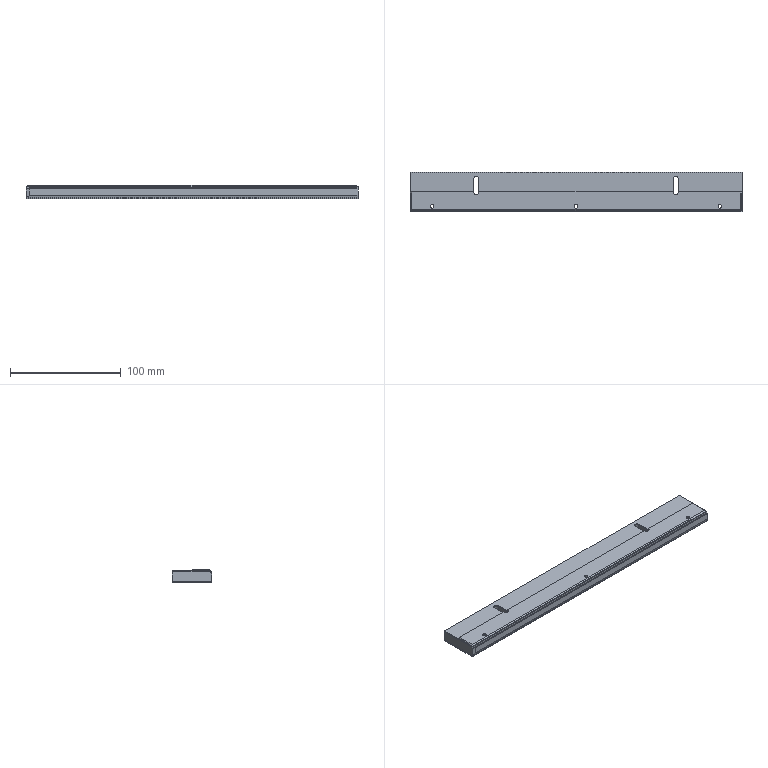CAM job | NX | 3-axis milling, drilling | part box 300 x 36 x 12 mm | stock box 305 x 41 x 15 mm
Tools:
number,name,description,diameter,corner_radius,flute_length,length,flutes
4,D4,平底铣刀-粗,4.0,0.0,25.0,75.0,2
6,D6,平底铣刀-粗,6.0,0.0,25.0,75.0,2
9,D10,平底铣刀-粗,10.0,0.0,35.0,75.0,2
11,D4-J,平底铣刀-精,4.0,0.0,50.0,75.0,2
7,D6-J,平底铣刀-精,6.0,0.0,25.0,75.0,2
10,D10-J,平底铣刀-精,10.0,0.0,35.0,75.0,2
17,D6R0.5,圆鼻刀-粗,6.0,0.5,50.0,75.0,2
2,D6倒角刀,倒角刀,6.0,0.0,3.0,25.0,2
21,M4X0.7,丝锥,3.3,0.0,35.0,50.0,2
13,ZT3.3,钻头,3.3,0.0,35.0,50.0,2
Operations:
program,operation,operation_type,tool,method,geometry_group,spindle_rpm,surface_speed,feed_per_tooth,feed_cut,feed_plunge,cut_length_mm,path_length_mm,cut_time_min,machine_time_min
D,顶面_COPY_COPY,FaceMilling,D10-J,侧刃精光-切深K-步距G,W-D,4500.0,1385.0,0.1667,1500.0,100.0,4781.035,5160.146,3.187,3.225
D,面铣自动飞面精光_COPY_COPY_COPY_1,FaceMilling,D10-J,侧刃精光-切深K-步距G,W-D,8000.0,251.327,0.0625,1000.0,100.0,2410.317,2466.317,2.41,2.416
D,底壁铣分层开粗-中_COPY_1,VolumeBased25DMillingOperation,D6,分层开粗-切深K-步距G,W-D,8000.0,150.792,0.1875,3000.0,100.0,4661.335,5306.774,1.554,1.618
D,打点-深0.8_2,Operation,D6倒角刀,NONE,W-D,8000.0,150.796,0.0312,500.0,90.0,5.4,332.808,0.0108,0.0435
D,通孔-M4螺纹底孔_2,Operation,ZT3.3,NONE,W-D,3000.0,30.536,0.05,300.0,90.0,48.0,418.008,0.16,0.197
D,钻倒角_1,Operation,D6倒角刀,METHOD,W-D,8000.0,150.796,0.0312,500.0,0.0,15.513,357.095,0.031,0.0652
D,通孔-攻牙M4_2,Operation,M4X0.7,METHOD,W-D,600.0,6.22,0.0006,0.7,90.0,42.0,406.008,60.0,60.036
D,底壁铣精光底面-中_COPY_1,VolumeBased25DMillingOperation,D6-J,精光步距切深关,W-D,8000.0,150.792,0.0625,1000.0,100.0,1838.862,1860.262,1.839,1.841
D,底壁铣精光侧面-中-选底面_COPY_1,VolumeBased25DMillingOperation,D6-J,侧刃精光-切深K-步距G,W-D,8000.0,150.792,0.0625,1000.0,100.0,312.168,334.568,0.3122,0.3144
D,底壁铣精光侧面-中_COPY,VolumeBased25DMillingOperation,D6-J,侧刃精光-切深K-步距G,W-D,8000.0,150.792,0.0625,1000.0,100.0,935.206,1617.172,0.9352,1.003
D,平面去毛刺6X45L_COPY_2,SurfaceContour,D6倒角刀,爬面_倒角-切深0-步距G,W-D,6500.0,122.519,0.1154,1500.0,100.0,753.227,1659.511,0.5022,0.5928
D,底壁铣倒角_COPY_2,VolumeBased25DMillingOperation,D6倒角刀,爬面_倒角-切深0-步距G,W-D,6500.0,122.519,0.1154,1500.0,100.0,349.496,408.896,0.233,0.2389
C,面铣自动飞面精光_COPY_COPY_COPY,FaceMilling,D10-J,侧刃精光-切深K-步距G,W-C,8000.0,251.327,0.0625,1000.0,100.0,4820.633,5253.341,4.821,4.864
C,面铣自动飞面精光_COPY_COPY,FaceMilling,D10-J,侧刃精光-切深K-步距G,W-C,8000.0,251.327,0.0625,1000.0,100.0,2410.317,2506.317,2.41,2.42
C,通腰槽粗_1,VolumeBased25DMillingOperation,D4,METHOD,W-C,10000.0,125.664,0.06,1200.0,100.0,2247.933,2645.634,1.873,1.913
C,腰槽精_1,VolumeBased25DMillingOperation,D4-J,METHOD,W-C,8000.0,100.531,0.0312,500.0,100.0,166.795,622.397,0.3336,0.3791
C,钻倒角_3,Operation,D6倒角刀,METHOD,W-C,8000.0,150.796,0.0312,500.0,0.0,15.45,356.969,0.0309,0.0651
C,平面去毛刺6X45L_COPY_1,SurfaceContour,D6倒角刀,爬面_倒角-切深0-步距G,W-C,6500.0,122.519,0.1154,1500.0,100.0,776.05,1373.78,0.5174,0.5771
C,等高精光往复爬面_COPY,ZLevelMilling,D6R0.5,等高爬面-切深K-步距G,W-C,8000.0,150.796,0.2812,4500.0,100.0,7843.439,7867.69,1.743,1.745
B,面铣自动飞面开粗_COPY,FaceMilling,D10-J,分层开粗-切深K-步距G,W-B,8000.0,251.327,0.1875,3000.0,100.0,11880.29,13292.228,3.96,4.101
B,面铣自动飞面精光_COPY,FaceMilling,D10-J,侧刃精光-切深K-步距G,W-B,8000.0,251.327,0.0625,1000.0,100.0,2410.317,2506.317,2.41,2.42
B,C0.3封闭铣廓倒角6X45L_COPY,PlanarMilling,D6倒角刀,爬面_倒角-切深0-步距G,W-B,7000.0,131.0,0.1071,1500.0,100.0,689.116,785.116,0.4594,0.469
A,顶面_1,FaceMilling,D10-J,侧刃精光-切深K-步距G,W-A,4500.0,1385.0,0.1667,1500.0,100.0,2390.518,2444.518,1.594,1.599
A,外形粗_2,VolumeBased25DMillingOperation,D10,METHOD,W-A,8000.0,251.327,0.375,6000.0,80.0,11962.495,12030.995,1.994,2.001
A,仅选体,SurfaceContour,D6倒角刀,METHOD,W-A,8000.0,150.796,0.1875,3000.0,100.0,687.815,741.616,0.2293,0.2347
A,外形半精_2,VolumeBased25DMillingOperation,D10-J,METHOD,W-A,9000.0,169.646,0.0667,1200.0,100.0,707.917,788.917,0.5899,0.598